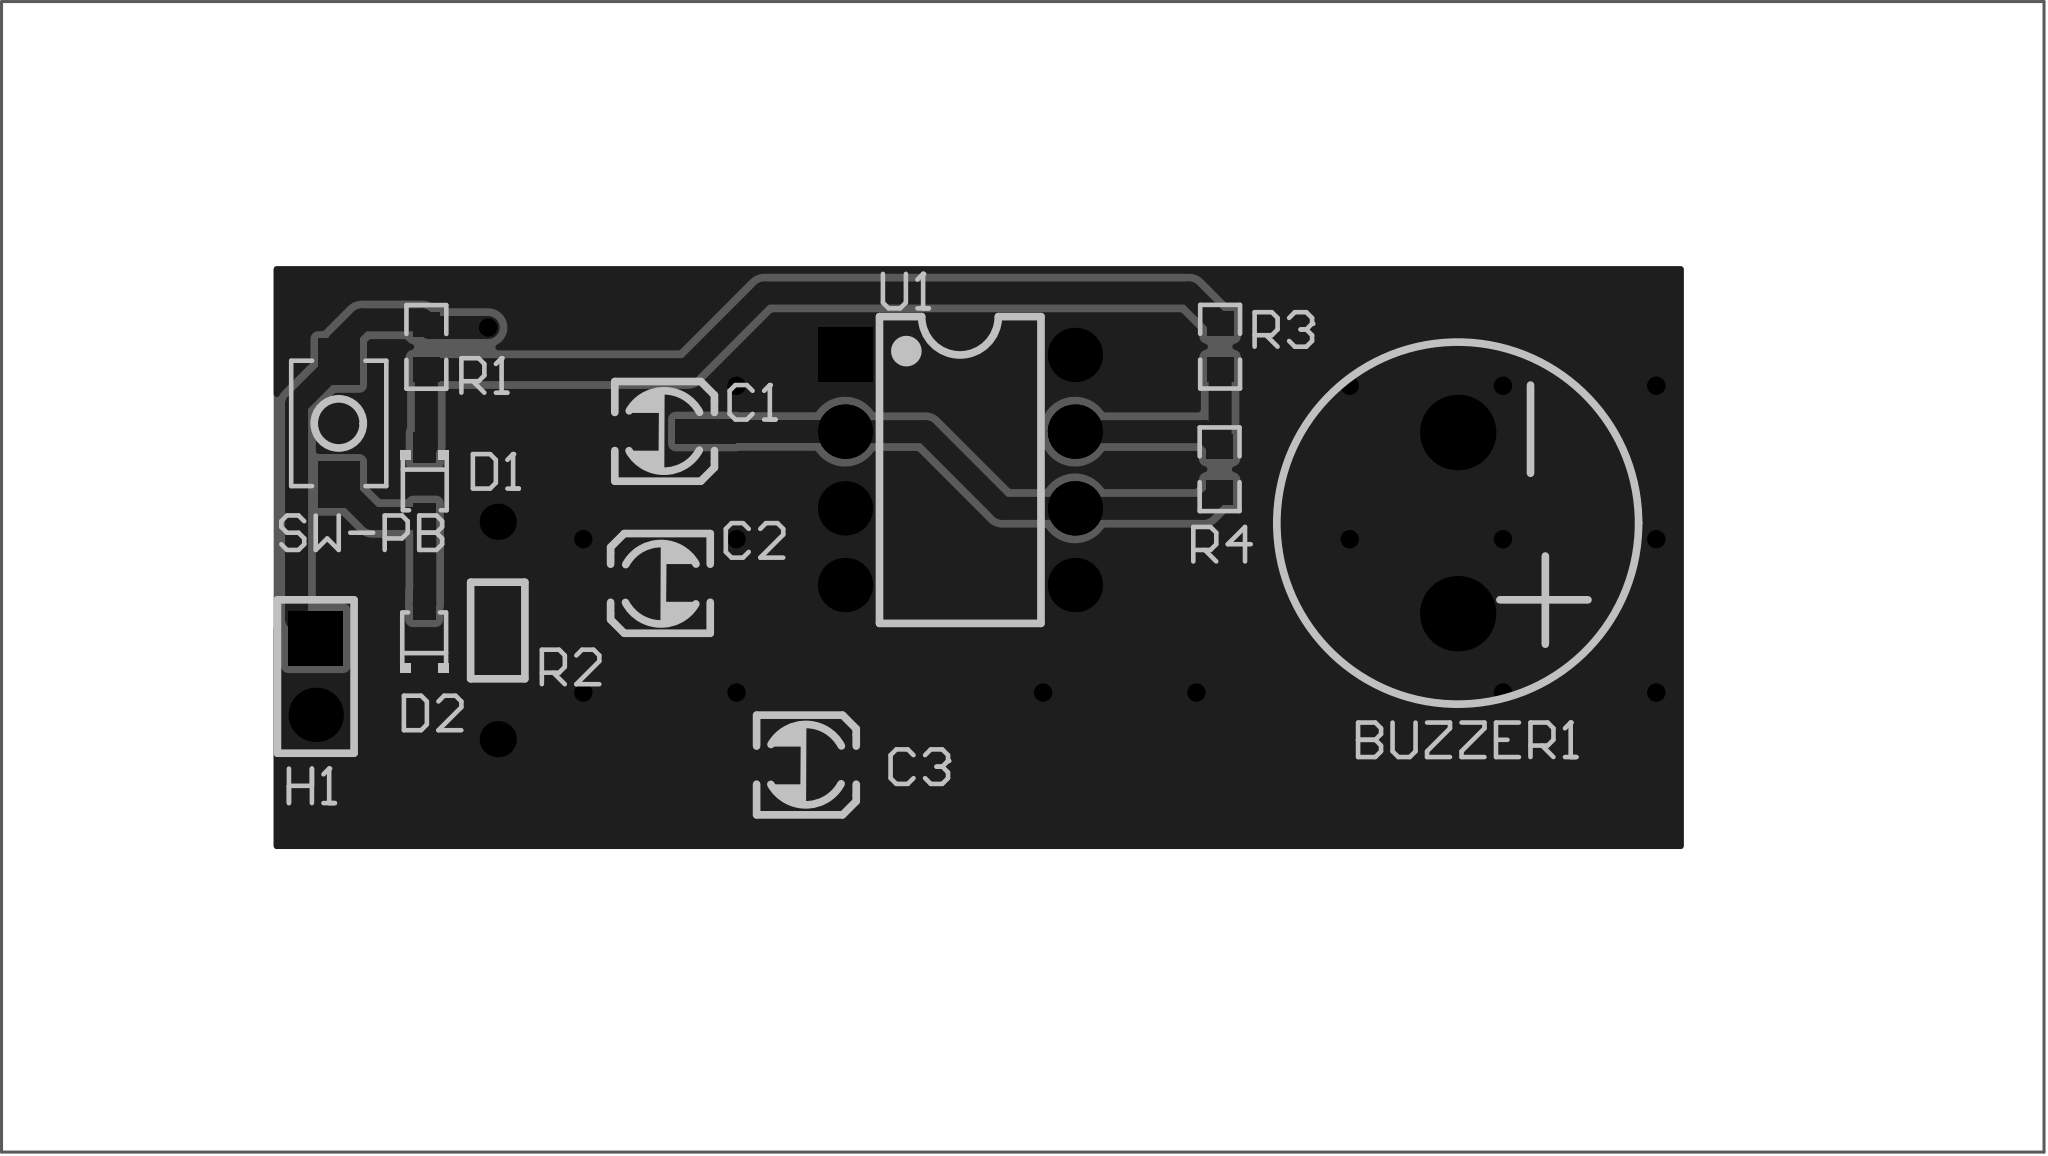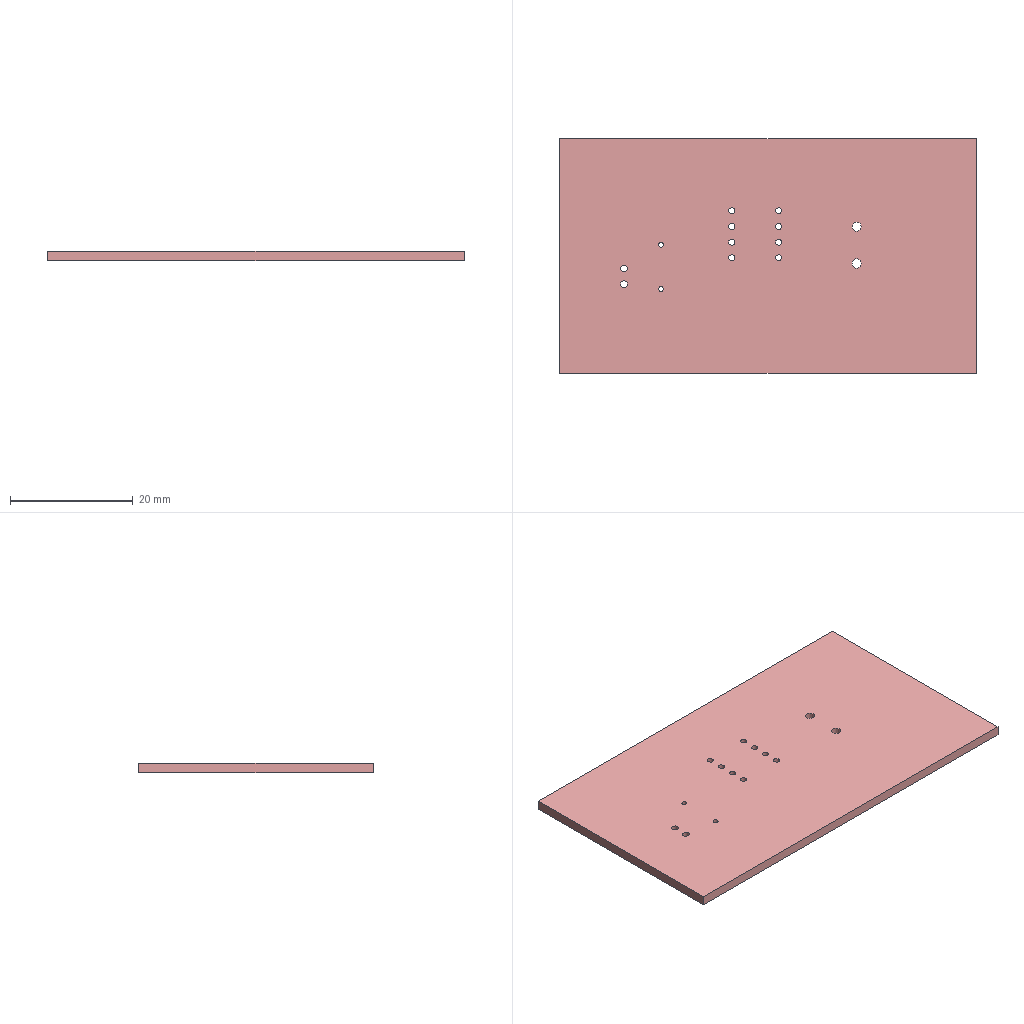Circuit board layout | Altium Designer | box 67.7 x 38.1 x 1.6 mm
Layer stack:
# Altium Designer layer stack of  (unit mm; dielectric type: 0 none, 1 core, 2 prepreg, 3 surface material)
index,name,kind,layer,copper_thickness_mm,dielectric_type,dielectric_thickness_mm,dielectric_material,dielectric_constant
0,Top Paste Mask Layer,other,,,,,,
1,Top Silkscreen Layer,other,,,,,,
2,Top Solder Mask Layer,dielectric,,,3,0.01,,3.3
3,Top Layer,copper,Top Layer,0.035,,,,
4,Dielectric1,dielectric,,,3,1.51,FR4,4.5
5,Bottom Layer,copper,Bottom Layer,0.035,,,,
6,Bottom Solder Mask Layer,dielectric,,,3,0.01,,3.3
7,Bottom Silkscreen Layer,other,,,,,,
8,Bottom Paste Mask Layer,other,,,,,,
# drill layer pairs: low layer,high layer
drill_pair,Top Layer,Bottom Layer
Part placement:
Designator,Comment,Layer,Footprint,Center-X(mm),Center-Y(mm),Rotation
BUZZER1,buzzer,TopLayer,BUZ-TH_BD12.0-P6.00-D0.9-RD,118.11,90.678,270
C1,0.01uF,TopLayer,C_Ele_SMD_3x5.4mm,91.826,93.712,0
C2,47uF,TopLayer,C_Ele_SMD_3x5.4mm,91.687,88.687,180
C3,47uF,TopLayer,C_Ele_SMD_3x5.4mm,96.525,82.663,0
D1,1N4148W,TopLayer,SOD-323_L1.8-W1.3-LS2.5-RD,83.877,92.004,270
D2,1N4148W,TopLayer,SOD-323_L1.8-W1.3-LS2.5-RD,83.857,86.819,90
H1,,TopLayer,HDR-TH_2P-P2.54-V-M-1,80.264,85.598,270
R1,30K,TopLayer,R0603,83.93,96.513,90
R2,47kΩ,TopLayer,Res_1/8W,86.296,87.122,270
R3,22K,TopLayer,R0603,110.236,96.52,90
R4,22K,TopLayer,R0603,110.219,92.461,90
SW-PB,,TopLayer,Key_SMD_3x4x2,81.026,93.98,90
U1,NE555N(XBLW),TopLayer,PDIP-8_L9.5-W6.4-P2.54-LS7.6-BL,101.615,92.437,270
Pad and via stacks:
# Altium Designer via and pad stacks of  (unit mm). Each distinct definition once, with the count of objects using it.
# via: kind,start_layer,end_layer,hole_mm,diameter_mm,mode(0 simple;1 top-mid-bottom;2 full stack),diameter_per_layer,count,example_net
# pad: kind,layer,hole_mm,hole_type(0 round;1 square;2 slot),plating,top_size,top_shape(1 round;2 rect;3 octagon;9 rounded rect),mid_size,bottom_size,mode,footprint,size_per_layer,count,example
pad,Multi-Layer,1.5,0,plated,2.5x2.5,1,2.5x2.5,2.5x2.5,0,BUZ-TH_BD12.0-P6.00-D0.9-RD,,2,BUZZER1.1
pad,Multi-Layer,1.1,0,plated,1.8x1.8,1,1.8x1.8,1.8x1.8,0,HDR-TH_2P-P2.54-V-M-1,,1,H1.2
pad,Multi-Layer,1.1,0,plated,1.8x1.8,2,1.8x1.8,1.8x1.8,0,HDR-TH_2P-P2.54-V-M-1,,1,H1.1
pad,Multi-Layer,0.8001,0,plated,1.199x1.199,1,1.199x1.199,1.199x1.199,0,Res_1/8W,,2,R2.1
pad,Multi-Layer,1,0,plated,1.8x1.8,1,1.8x1.8,1.8x1.8,0,PDIP-8_L9.5-W6.4-P2.54-LS7.6-BL,,7,U1.8
pad,Multi-Layer,1,0,plated,1.8x1.8,2,1.8x1.8,1.8x1.8,0,PDIP-8_L9.5-W6.4-P2.54-LS7.6-BL,,1,U1.1
pad,Top Layer,0,0,plated,1.999x0.8001,2,1.999x0.8001,1.999x0.8001,0,C_Ele_SMD_3x5.4mm,,6,C1.1
pad,Top Layer,0,0,plated,1x0.75,2,1x0.75,1x0.75,0,SOD-323_L1.8-W1.3-LS2.5-RD,,4,D1.2
pad,Top Layer,0,0,plated,0.8065x0.864,2,0.8065x0.864,0.8065x0.864,0,R0603,,6,R1.2
pad,Top Layer,0,0,plated,1.53x1.36,2,1.53x1.36,1.53x1.36,0,Key_SMD_3x4x2,,2,SW-PB.1
via,Top Layer,Bottom Layer,0.3048,0.61,0,,16,$1N3
Copper pours:
name,layer,net,type(0 solid;1 hatched;2 none)
Top Layer-GND,Top Layer,GND,0
Bottom Layer-GND,Bottom Layer,GND,0